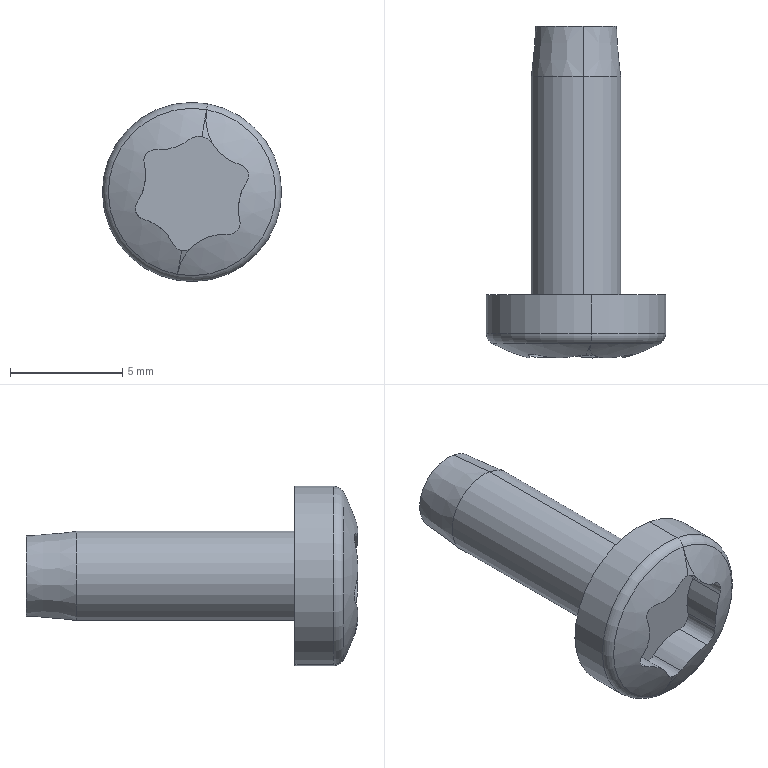Part | SolidWorks | features BaseBody 1 | 1 solid | 27 faces | box 8 x 14.81 x 8 mm | volume 243.858 mm3 | cylinder 16 | sphere 4 | plane 3 | torus 2 | cone 2 | commonest cylinder face diameters 4.272 x6 1 x5 4 x2 8 x2 1.5 x1
STEP:
#1=CARTESIAN_POINT('',(2057.198,-49.401,812.67));
#2=VERTEX_POINT('',#1);
#3=CARTESIAN_POINT('',(2056.608,-49.458,812.525));
#4=VERTEX_POINT('',#3);
#5=CARTESIAN_POINT('',(2057.198,-49.401,812.67));
#6=CARTESIAN_POINT('',(2057.147,-49.401,812.679));
#7=CARTESIAN_POINT('',(2057.043,-49.404,812.687));
#8=CARTESIAN_POINT('',(2056.888,-49.415,812.666));
#9=CARTESIAN_POINT('',(2056.74,-49.433,812.613));
#10=CARTESIAN_POINT('',(2056.65,-49.449,812.558));
#11=CARTESIAN_POINT('',(2056.608,-49.458,812.525));
#12=B_SPLINE_CURVE_WITH_KNOTS('',3,(#5,#6,#7,#8,#9,#10,#11),.UNSPECIFIED.,.F.,.F.,(4,1,1,1,4),(0.5,0.625,0.75,0.875,1.),.UNSPECIFIED.);
#13=EDGE_CURVE('',#2,#4,#12,.T.);
#14=ORIENTED_EDGE('',*,*,#13,.F.);
#15=CARTESIAN_POINT('',(2057.406,-48.898,813.843));
#16=VERTEX_POINT('',#15);
#17=CARTESIAN_POINT('',(2056.759,-41.805,810.2));
#18=DIRECTION('',(-0.9846,0.,0.1747));
#19=DIRECTION('',(0.1747,0.,0.9846));
#20=AXIS2_PLACEMENT_3D('',#17,#18,#19);
#21=CIRCLE('',#20,8.);
#22=EDGE_CURVE('',#2,#16,#21,.T.);
#23=ORIENTED_EDGE('',*,*,#22,.T.);
#24=CARTESIAN_POINT('',(2057.412,-48.88,813.876));
#25=VERTEX_POINT('',#24);
#26=CARTESIAN_POINT('',(2056.759,-41.805,810.2));
#27=DIRECTION('',(0.9846,0.,-0.1747));
#28=DIRECTION('',(0.08155,-0.8844,0.4595));
#29=AXIS2_PLACEMENT_3D('',#26,#27,#28);
#30=CIRCLE('',#29,8.);
#31=EDGE_CURVE('',#25,#16,#30,.T.);
#32=ORIENTED_EDGE('',*,*,#31,.F.);
#33=CARTESIAN_POINT('',(2056.107,-48.88,806.524));
#34=VERTEX_POINT('',#33);
#35=CARTESIAN_POINT('',(2056.759,-48.88,810.2));
#36=DIRECTION('',(0.,1.,0.));
#37=DIRECTION('',(-0.1747,0.,-0.9846));
#38=AXIS2_PLACEMENT_3D('',#35,#36,#37);
#39=CIRCLE('',#38,3.733);
#40=EDGE_CURVE('',#34,#25,#39,.T.);
#41=ORIENTED_EDGE('',*,*,#40,.F.);
#42=CARTESIAN_POINT('',(2056.113,-48.898,806.557));
#43=VERTEX_POINT('',#42);
#44=CARTESIAN_POINT('',(2056.759,-41.805,810.2));
#45=DIRECTION('',(0.9846,0.,-0.1747));
#46=DIRECTION('',(-0.08155,-0.8844,-0.4595));
#47=AXIS2_PLACEMENT_3D('',#44,#45,#46);
#48=CIRCLE('',#47,8.);
#49=EDGE_CURVE('',#43,#34,#48,.T.);
#50=ORIENTED_EDGE('',*,*,#49,.F.);
#51=CARTESIAN_POINT('',(2056.295,-49.351,807.585));
#52=VERTEX_POINT('',#51);
#53=CARTESIAN_POINT('',(2056.759,-41.805,810.2));
#54=DIRECTION('',(0.9846,0.,-0.1747));
#55=DIRECTION('',(-0.1747,0.,-0.9846));
#56=AXIS2_PLACEMENT_3D('',#53,#54,#55);
#57=CIRCLE('',#56,8.);
#58=EDGE_CURVE('',#52,#43,#57,.T.);
#59=ORIENTED_EDGE('',*,*,#58,.F.);
#60=CARTESIAN_POINT('',(2055.933,-49.41,807.86));
#61=VERTEX_POINT('',#60);
#62=CARTESIAN_POINT('',(2056.295,-49.351,807.585));
#63=CARTESIAN_POINT('',(2056.257,-49.351,807.592));
#64=CARTESIAN_POINT('',(2056.182,-49.354,807.615));
#65=CARTESIAN_POINT('',(2056.08,-49.366,807.674));
#66=CARTESIAN_POINT('',(2055.994,-49.384,807.756));
#67=CARTESIAN_POINT('',(2055.95,-49.401,807.824));
#68=CARTESIAN_POINT('',(2055.933,-49.41,807.86));
#69=B_SPLINE_CURVE_WITH_KNOTS('',3,(#62,#63,#64,#65,#66,#67,#68),.UNSPECIFIED.,.F.,.F.,(4,1,1,1,4),(0.5,0.625,0.75,0.875,1.),.UNSPECIFIED.);
#70=EDGE_CURVE('',#52,#61,#69,.T.);
#71=ORIENTED_EDGE('',*,*,#70,.T.);
#72=CARTESIAN_POINT('',(2054.596,-49.41,808.984));
#73=VERTEX_POINT('',#72);
#74=CARTESIAN_POINT('',(2055.933,-49.41,807.86));
#75=CARTESIAN_POINT('',(2055.868,-49.445,807.994));
#76=CARTESIAN_POINT('',(2055.79,-49.47,808.12));
#77=CARTESIAN_POINT('',(2055.606,-49.505,808.357));
#78=CARTESIAN_POINT('',(2055.5,-49.514,808.468));
#79=CARTESIAN_POINT('',(2055.27,-49.515,808.661));
#80=CARTESIAN_POINT('',(2055.144,-49.506,808.746));
#81=CARTESIAN_POINT('',(2054.877,-49.47,808.888));
#82=CARTESIAN_POINT('',(2054.739,-49.445,808.943));
#83=CARTESIAN_POINT('',(2054.596,-49.41,808.984));
#84=B_SPLINE_CURVE_WITH_KNOTS('',3,(#74,#75,#76,#77,#78,#79,#80,#81,#82,#83),.UNSPECIFIED.,.F.,.F.,(4,2,2,2,4),(0.,0.0004513,0.0009026,0.001354,0.001805),.UNSPECIFIED.);
#85=EDGE_CURVE('',#61,#73,#84,.T.);
#86=ORIENTED_EDGE('',*,*,#85,.T.);
#87=CARTESIAN_POINT('',(2054.32,-49.41,809.746));
#88=VERTEX_POINT('',#87);
#89=CARTESIAN_POINT('',(2054.596,-49.41,808.984));
#90=CARTESIAN_POINT('',(2054.557,-49.401,808.995));
#91=CARTESIAN_POINT('',(2054.483,-49.384,809.026));
#92=CARTESIAN_POINT('',(2054.388,-49.366,809.097));
#93=CARTESIAN_POINT('',(2054.312,-49.354,809.188));
#94=CARTESIAN_POINT('',(2054.259,-49.35,809.293));
#95=CARTESIAN_POINT('',(2054.232,-49.354,809.407));
#96=CARTESIAN_POINT('',(2054.232,-49.366,809.526));
#97=CARTESIAN_POINT('',(2054.26,-49.384,809.641));
#98=CARTESIAN_POINT('',(2054.297,-49.401,809.713));
#99=CARTESIAN_POINT('',(2054.32,-49.41,809.746));
#100=B_SPLINE_CURVE_WITH_KNOTS('',3,(#89,#90,#91,#92,#93,#94,#95,#96,#97,#98,#99),.UNSPECIFIED.,.F.,.F.,(4,1,1,1,1,1,1,1,4),(0.,0.125,0.25,0.375,0.5,0.625,0.75,0.875,1.),.UNSPECIFIED.);
#101=EDGE_CURVE('',#73,#88,#100,.T.);
#102=ORIENTED_EDGE('',*,*,#101,.T.);
#103=CARTESIAN_POINT('',(2054.625,-49.41,811.465));
#104=VERTEX_POINT('',#103);
#105=CARTESIAN_POINT('',(2054.32,-49.41,809.746));
#106=CARTESIAN_POINT('',(2054.403,-49.445,809.869));
#107=CARTESIAN_POINT('',(2054.473,-49.47,810.));
#108=CARTESIAN_POINT('',(2054.587,-49.505,810.277));
#109=CARTESIAN_POINT('',(2054.63,-49.514,810.424));
#110=CARTESIAN_POINT('',(2054.682,-49.515,810.721));
#111=CARTESIAN_POINT('',(2054.693,-49.506,810.872));
#112=CARTESIAN_POINT('',(2054.682,-49.47,811.174));
#113=CARTESIAN_POINT('',(2054.661,-49.445,811.321));
#114=CARTESIAN_POINT('',(2054.625,-49.41,811.465));
#115=B_SPLINE_CURVE_WITH_KNOTS('',3,(#105,#106,#107,#108,#109,#110,#111,#112,#113,#114),.UNSPECIFIED.,.F.,.F.,(4,2,2,2,4),(0.,0.0004513,0.0009026,0.001354,0.001805),.UNSPECIFIED.);
#116=EDGE_CURVE('',#88,#104,#115,.T.);
#117=ORIENTED_EDGE('',*,*,#116,.T.);
#118=CARTESIAN_POINT('',(2055.146,-49.41,812.086));
#119=VERTEX_POINT('',#118);
#120=CARTESIAN_POINT('',(2054.625,-49.41,811.465));
#121=CARTESIAN_POINT('',(2054.615,-49.401,811.504));
#122=CARTESIAN_POINT('',(2054.605,-49.384,811.584));
#123=CARTESIAN_POINT('',(2054.619,-49.366,811.702));
#124=CARTESIAN_POINT('',(2054.659,-49.354,811.813));
#125=CARTESIAN_POINT('',(2054.724,-49.35,811.912));
#126=CARTESIAN_POINT('',(2054.81,-49.354,811.992));
#127=CARTESIAN_POINT('',(2054.912,-49.366,812.051));
#128=CARTESIAN_POINT('',(2055.026,-49.384,812.085));
#129=CARTESIAN_POINT('',(2055.106,-49.401,812.089));
#130=CARTESIAN_POINT('',(2055.146,-49.41,812.086));
#131=B_SPLINE_CURVE_WITH_KNOTS('',3,(#120,#121,#122,#123,#124,#125,#126,#127,#128,#129,#130),.UNSPECIFIED.,.F.,.F.,(4,1,1,1,1,1,1,1,4),(0.,0.125,0.25,0.375,0.5,0.625,0.75,0.875,1.),.UNSPECIFIED.);
#132=EDGE_CURVE('',#104,#119,#131,.T.);
#133=ORIENTED_EDGE('',*,*,#132,.T.);
#134=CARTESIAN_POINT('',(2055.146,-49.41,812.086));
#135=CARTESIAN_POINT('',(2055.215,-49.426,812.081));
#136=CARTESIAN_POINT('',(2055.35,-49.454,812.077));
#137=CARTESIAN_POINT('',(2055.547,-49.484,812.091));
#138=CARTESIAN_POINT('',(2055.738,-49.504,812.122));
#139=CARTESIAN_POINT('',(2055.925,-49.514,812.17));
#140=CARTESIAN_POINT('',(2056.108,-49.515,812.234));
#141=CARTESIAN_POINT('',(2056.283,-49.506,812.315));
#142=CARTESIAN_POINT('',(2056.45,-49.488,812.411));
#143=CARTESIAN_POINT('',(2056.557,-49.469,812.486));
#144=CARTESIAN_POINT('',(2056.608,-49.458,812.525));
#145=B_SPLINE_CURVE_WITH_KNOTS('',3,(#134,#135,#136,#137,#138,#139,#140,#141,#142,#143,#144),.UNSPECIFIED.,.F.,.F.,(4,1,1,1,1,1,1,1,4),(0.,0.125,0.25,0.375,0.5,0.625,0.75,0.875,1.),.UNSPECIFIED.);
#146=EDGE_CURVE('',#119,#4,#145,.T.);
#147=ORIENTED_EDGE('',*,*,#146,.T.);
#148=EDGE_LOOP('',(#14,#23,#32,#41,#50,#59,#71,#86,#102,#117,#133,#147));
#149=FACE_OUTER_BOUND('',#148,.T.);
#150=CARTESIAN_POINT('',(2056.759,-41.805,810.2));
#151=DIRECTION('',(-0.9846,0.,0.1747));
#152=DIRECTION('',(-0.1747,0.,-0.9846));
#153=AXIS2_PLACEMENT_3D('',#150,#151,#152);
#154=SPHERICAL_SURFACE('',#153,8.);
#155=ADVANCED_FACE('',(#149),#154,.T.);
#156=CARTESIAN_POINT('',(2056.73,-49.41,807.718));
#157=VERTEX_POINT('',#156);
#158=CARTESIAN_POINT('',(2056.73,-49.41,807.718));
#159=CARTESIAN_POINT('',(2056.702,-49.401,807.69));
#160=CARTESIAN_POINT('',(2056.638,-49.384,807.642));
#161=CARTESIAN_POINT('',(2056.529,-49.366,807.595));
#162=CARTESIAN_POINT('',(2056.412,-49.354,807.574));
#163=CARTESIAN_POINT('',(2056.334,-49.351,807.579));
#164=CARTESIAN_POINT('',(2056.295,-49.351,807.585));
#165=B_SPLINE_CURVE_WITH_KNOTS('',3,(#158,#159,#160,#161,#162,#163,#164),.UNSPECIFIED.,.F.,.F.,(4,1,1,1,4),(0.,0.125,0.25,0.375,0.5),.UNSPECIFIED.);
#166=EDGE_CURVE('',#157,#52,#165,.T.);
#167=ORIENTED_EDGE('',*,*,#166,.T.);
#168=ORIENTED_EDGE('',*,*,#58,.T.);
#169=CARTESIAN_POINT('',(2056.73,-49.41,807.718));
#170=CARTESIAN_POINT('',(2056.679,-49.394,807.669));
#171=CARTESIAN_POINT('',(2056.578,-49.356,807.561));
#172=CARTESIAN_POINT('',(2056.434,-49.282,807.37));
#173=CARTESIAN_POINT('',(2056.3,-49.185,807.141));
#174=CARTESIAN_POINT('',(2056.186,-49.06,806.872));
#175=CARTESIAN_POINT('',(2056.132,-48.956,806.666));
#176=CARTESIAN_POINT('',(2056.113,-48.898,806.557));
#177=B_SPLINE_CURVE_WITH_KNOTS('',3,(#169,#170,#171,#172,#173,#174,#175,#176),.UNSPECIFIED.,.F.,.F.,(4,1,1,1,1,4),(0.,0.2,0.4,0.6,0.8,1.),.UNSPECIFIED.);
#178=EDGE_CURVE('',#157,#43,#177,.T.);
#179=ORIENTED_EDGE('',*,*,#178,.F.);
#180=EDGE_LOOP('',(#167,#168,#179));
#181=FACE_OUTER_BOUND('',#180,.T.);
#182=CARTESIAN_POINT('',(2056.759,-41.805,810.2));
#183=DIRECTION('',(-0.9846,0.,0.1747));
#184=DIRECTION('',(-0.1747,0.,-0.9846));
#185=AXIS2_PLACEMENT_3D('',#182,#183,#184);
#186=SPHERICAL_SURFACE('',#185,8.);
#187=ADVANCED_FACE('',(#181),#186,.T.);
#188=CARTESIAN_POINT('',(2056.06,-46.705,806.261));
#189=VERTEX_POINT('',#188);
#190=CARTESIAN_POINT('',(2057.458,-46.705,814.138));
#191=VERTEX_POINT('',#190);
#192=CARTESIAN_POINT('',(2056.759,-46.705,810.2));
#193=DIRECTION('',(0.,-1.,0.));
#194=DIRECTION('',(-0.1747,0.,-0.9846));
#195=AXIS2_PLACEMENT_3D('',#192,#193,#194);
#196=CIRCLE('',#195,4.);
#197=EDGE_CURVE('',#189,#191,#196,.T.);
#198=ORIENTED_EDGE('',*,*,#197,.F.);
#199=CARTESIAN_POINT('',(2056.759,-46.705,810.2));
#200=DIRECTION('',(0.,1.,0.));
#201=DIRECTION('',(-0.1747,0.,-0.9846));
#202=AXIS2_PLACEMENT_3D('',#199,#200,#201);
#203=CIRCLE('',#202,4.);
#204=EDGE_CURVE('',#189,#191,#203,.T.);
#205=ORIENTED_EDGE('',*,*,#204,.T.);
#206=EDGE_LOOP('',(#198,#205));
#207=FACE_OUTER_BOUND('',#206,.T.);
#208=CARTESIAN_POINT('',(2056.41,-46.705,808.231));
#209=VERTEX_POINT('',#208);
#210=CARTESIAN_POINT('',(2057.109,-46.705,812.169));
#211=VERTEX_POINT('',#210);
#212=CARTESIAN_POINT('',(2056.759,-46.705,810.2));
#213=DIRECTION('',(0.,1.,0.));
#214=DIRECTION('',(-0.1747,0.,-0.9846));
#215=AXIS2_PLACEMENT_3D('',#212,#213,#214);
#216=CIRCLE('',#215,2.);
#217=EDGE_CURVE('',#209,#211,#216,.T.);
#218=ORIENTED_EDGE('',*,*,#217,.F.);
#219=CARTESIAN_POINT('',(2056.759,-46.705,810.2));
#220=DIRECTION('',(0.,-1.,0.));
#221=DIRECTION('',(-0.1747,0.,-0.9846));
#222=AXIS2_PLACEMENT_3D('',#219,#220,#221);
#223=CIRCLE('',#222,2.);
#224=EDGE_CURVE('',#209,#211,#223,.T.);
#225=ORIENTED_EDGE('',*,*,#224,.T.);
#226=EDGE_LOOP('',(#218,#225));
#227=FACE_BOUND('',#226,.T.);
#228=CARTESIAN_POINT('',(2056.759,-46.705,810.2));
#229=DIRECTION('',(0.,1.,0.));
#230=DIRECTION('',(-0.1747,0.,-0.9846));
#231=AXIS2_PLACEMENT_3D('',#228,#229,#230);
#232=PLANE('',#231);
#233=ADVANCED_FACE('',(#207,#227),#232,.T.);
#234=CARTESIAN_POINT('',(2056.06,-48.438,806.261));
#235=VERTEX_POINT('',#234);
#236=CARTESIAN_POINT('',(2057.458,-48.438,814.138));
#237=VERTEX_POINT('',#236);
#238=CARTESIAN_POINT('',(2056.759,-48.438,810.2));
#239=DIRECTION('',(0.,1.,0.));
#240=DIRECTION('',(-0.1747,0.,-0.9846));
#241=AXIS2_PLACEMENT_3D('',#238,#239,#240);
#242=CIRCLE('',#241,4.);
#243=EDGE_CURVE('',#235,#237,#242,.T.);
#244=ORIENTED_EDGE('',*,*,#243,.T.);
#245=CARTESIAN_POINT('',(2057.458,-46.705,814.138));
#246=DIRECTION('',(0.,1.,0.));
#247=VECTOR('',#246,1000.);
#248=LINE('',#245,#247);
#249=EDGE_CURVE('',#237,#191,#248,.T.);
#250=ORIENTED_EDGE('',*,*,#249,.T.);
#251=ORIENTED_EDGE('',*,*,#204,.F.);
#252=CARTESIAN_POINT('',(2056.06,-46.705,806.261));
#253=DIRECTION('',(0.,-1.,0.));
#254=VECTOR('',#253,1000.);
#255=LINE('',#252,#254);
#256=EDGE_CURVE('',#189,#235,#255,.T.);
#257=ORIENTED_EDGE('',*,*,#256,.T.);
#258=EDGE_LOOP('',(#244,#250,#251,#257));
#259=FACE_OUTER_BOUND('',#258,.T.);
#260=CARTESIAN_POINT('',(2056.759,-50.56,810.2));
#261=DIRECTION('',(0.,1.,0.));
#262=DIRECTION('',(-0.1747,0.,-0.9846));
#263=AXIS2_PLACEMENT_3D('',#260,#261,#262);
#264=CYLINDRICAL_SURFACE('',#263,4.);
#265=ADVANCED_FACE('',(#259),#264,.T.);
#266=ORIENTED_EDGE('',*,*,#197,.T.);
#267=ORIENTED_EDGE('',*,*,#249,.F.);
#268=CARTESIAN_POINT('',(2056.759,-48.438,810.2));
#269=DIRECTION('',(0.,-1.,0.));
#270=DIRECTION('',(-0.1747,0.,-0.9846));
#271=AXIS2_PLACEMENT_3D('',#268,#269,#270);
#272=CIRCLE('',#271,4.);
#273=EDGE_CURVE('',#235,#237,#272,.T.);
#274=ORIENTED_EDGE('',*,*,#273,.F.);
#275=ORIENTED_EDGE('',*,*,#256,.F.);
#276=EDGE_LOOP('',(#266,#267,#274,#275));
#277=FACE_OUTER_BOUND('',#276,.T.);
#278=CARTESIAN_POINT('',(2056.759,-50.56,810.2));
#279=DIRECTION('',(0.,1.,0.));
#280=DIRECTION('',(-0.1747,0.,-0.9846));
#281=AXIS2_PLACEMENT_3D('',#278,#279,#280);
#282=CYLINDRICAL_SURFACE('',#281,4.);
#283=ADVANCED_FACE('',(#277),#282,.T.);
#284=ORIENTED_EDGE('',*,*,#273,.T.);
#285=CARTESIAN_POINT('',(2057.371,-48.438,813.646));
#286=DIRECTION('',(-0.9846,0.,0.1747));
#287=DIRECTION('',(0.1747,0.,0.9846));
#288=AXIS2_PLACEMENT_3D('',#285,#286,#287);
#289=CIRCLE('',#288,0.5);
#290=EDGE_CURVE('',#25,#237,#289,.T.);
#291=ORIENTED_EDGE('',*,*,#290,.F.);
#292=CARTESIAN_POINT('',(2056.759,-48.88,810.2));
#293=DIRECTION('',(0.,-1.,0.));
#294=DIRECTION('',(-0.1747,0.,-0.9846));
#295=AXIS2_PLACEMENT_3D('',#292,#293,#294);
#296=CIRCLE('',#295,3.733);
#297=EDGE_CURVE('',#34,#25,#296,.T.);
#298=ORIENTED_EDGE('',*,*,#297,.F.);
#299=CARTESIAN_POINT('',(2056.148,-48.438,806.754));
#300=DIRECTION('',(-0.9846,0.,0.1747));
#301=DIRECTION('',(-0.1747,0.,-0.9846));
#302=AXIS2_PLACEMENT_3D('',#299,#300,#301);
#303=CIRCLE('',#302,0.5);
#304=EDGE_CURVE('',#235,#34,#303,.T.);
#305=ORIENTED_EDGE('',*,*,#304,.F.);
#306=EDGE_LOOP('',(#284,#291,#298,#305));
#307=FACE_OUTER_BOUND('',#306,.T.);
#308=CARTESIAN_POINT('',(2056.759,-48.438,810.2));
#309=DIRECTION('',(0.,1.,0.));
#310=DIRECTION('',(-0.1747,0.,-0.9846));
#311=AXIS2_PLACEMENT_3D('',#308,#309,#310);
#312=TOROIDAL_SURFACE('',#311,3.5,0.5);
#313=ADVANCED_FACE('',(#307),#312,.T.);
#314=ORIENTED_EDGE('',*,*,#40,.T.);
#315=ORIENTED_EDGE('',*,*,#290,.T.);
#316=ORIENTED_EDGE('',*,*,#243,.F.);
#317=ORIENTED_EDGE('',*,*,#304,.T.);
#318=EDGE_LOOP('',(#314,#315,#316,#317));
#319=FACE_OUTER_BOUND('',#318,.T.);
#320=CARTESIAN_POINT('',(2056.759,-48.438,810.2));
#321=DIRECTION('',(0.,1.,0.));
#322=DIRECTION('',(-0.1747,0.,-0.9846));
#323=AXIS2_PLACEMENT_3D('',#320,#321,#322);
#324=TOROIDAL_SURFACE('',#323,3.5,0.5);
#325=ADVANCED_FACE('',(#319),#324,.T.);
#326=ORIENTED_EDGE('',*,*,#22,.F.);
#327=CARTESIAN_POINT('',(2057.701,-49.458,812.331));
#328=VERTEX_POINT('',#327);
#329=CARTESIAN_POINT('',(2057.701,-49.458,812.331));
#330=CARTESIAN_POINT('',(2057.673,-49.449,812.376));
#331=CARTESIAN_POINT('',(2057.608,-49.433,812.459));
#332=CARTESIAN_POINT('',(2057.487,-49.415,812.559));
#333=CARTESIAN_POINT('',(2057.349,-49.404,812.633));
#334=CARTESIAN_POINT('',(2057.249,-49.401,812.661));
#335=CARTESIAN_POINT('',(2057.198,-49.401,812.67));
#336=B_SPLINE_CURVE_WITH_KNOTS('',3,(#329,#330,#331,#332,#333,#334,#335),.UNSPECIFIED.,.F.,.F.,(4,1,1,1,4),(0.,0.125,0.25,0.375,0.5),.UNSPECIFIED.);
#337=EDGE_CURVE('',#328,#2,#336,.T.);
#338=ORIENTED_EDGE('',*,*,#337,.F.);
#339=CARTESIAN_POINT('',(2057.406,-48.898,813.843));
#340=CARTESIAN_POINT('',(2057.387,-48.953,813.738));
#341=CARTESIAN_POINT('',(2057.367,-49.054,813.534));
#342=CARTESIAN_POINT('',(2057.379,-49.179,813.244));
#343=CARTESIAN_POINT('',(2057.425,-49.279,812.979));
#344=CARTESIAN_POINT('',(2057.496,-49.356,812.741));
#345=CARTESIAN_POINT('',(2057.59,-49.416,812.522));
#346=CARTESIAN_POINT('',(2057.662,-49.446,812.393));
#347=CARTESIAN_POINT('',(2057.701,-49.458,812.331));
#348=B_SPLINE_CURVE_WITH_KNOTS('',3,(#339,#340,#341,#342,#343,#344,#345,#346,#347),.UNSPECIFIED.,.F.,.F.,(4,1,1,1,1,1,4),(0.,0.1667,0.3333,0.5,0.6667,0.8333,1.),.UNSPECIFIED.);
#349=EDGE_CURVE('',#16,#328,#348,.T.);
#350=ORIENTED_EDGE('',*,*,#349,.F.);
#351=EDGE_LOOP('',(#326,#338,#350));
#352=FACE_OUTER_BOUND('',#351,.T.);
#353=CARTESIAN_POINT('',(2056.759,-41.805,810.2));
#354=DIRECTION('',(-0.9846,0.,0.1747));
#355=DIRECTION('',(-0.1747,0.,-0.9846));
#356=AXIS2_PLACEMENT_3D('',#353,#354,#355);
#357=SPHERICAL_SURFACE('',#356,8.);
#358=ADVANCED_FACE('',(#352),#357,.T.);
#359=CARTESIAN_POINT('',(2054.32,-47.705,809.746));
#360=VERTEX_POINT('',#359);
#361=CARTESIAN_POINT('',(2054.625,-47.705,811.465));
#362=VERTEX_POINT('',#361);
#363=CARTESIAN_POINT('',(2052.553,-47.705,810.946));
#364=DIRECTION('',(0.,-1.,0.));
#365=DIRECTION('',(0.8272,0.,-0.562));
#366=AXIS2_PLACEMENT_3D('',#363,#364,#365);
#367=CIRCLE('',#366,2.136);
#368=EDGE_CURVE('',#360,#362,#367,.T.);
#369=ORIENTED_EDGE('',*,*,#368,.T.);
#370=CARTESIAN_POINT('',(2054.625,-49.41,811.465));
#371=DIRECTION('',(0.,1.,0.));
#372=VECTOR('',#371,1000.);
#373=LINE('',#370,#372);
#374=EDGE_CURVE('',#104,#362,#373,.T.);
#375=ORIENTED_EDGE('',*,*,#374,.F.);
#376=ORIENTED_EDGE('',*,*,#116,.F.);
#377=CARTESIAN_POINT('',(2054.32,-49.41,809.746));
#378=DIRECTION('',(0.,1.,0.));
#379=VECTOR('',#378,1000.);
#380=LINE('',#377,#379);
#381=EDGE_CURVE('',#88,#360,#380,.T.);
#382=ORIENTED_EDGE('',*,*,#381,.T.);
#383=EDGE_LOOP('',(#369,#375,#376,#382));
#384=FACE_OUTER_BOUND('',#383,.T.);
#385=CARTESIAN_POINT('',(2052.553,-47.705,810.946));
#386=DIRECTION('',(0.,1.,0.));
#387=DIRECTION('',(-0.1747,0.,-0.9846));
#388=AXIS2_PLACEMENT_3D('',#385,#386,#387);
#389=CYLINDRICAL_SURFACE('',#388,2.136);
#390=ADVANCED_FACE('',(#384),#389,.T.);
#391=CARTESIAN_POINT('',(2054.596,-47.705,808.984));
#392=VERTEX_POINT('',#391);
#393=CARTESIAN_POINT('',(2054.733,-47.705,809.465));
#394=DIRECTION('',(0.,1.,0.));
#395=DIRECTION('',(-0.2746,0.,-0.9616));
#396=AXIS2_PLACEMENT_3D('',#393,#394,#395);
#397=CIRCLE('',#396,0.5);
#398=EDGE_CURVE('',#392,#360,#397,.T.);
#399=ORIENTED_EDGE('',*,*,#398,.T.);
#400=ORIENTED_EDGE('',*,*,#381,.F.);
#401=ORIENTED_EDGE('',*,*,#101,.F.);
#402=CARTESIAN_POINT('',(2054.596,-49.41,808.984));
#403=DIRECTION('',(0.,1.,0.));
#404=VECTOR('',#403,1000.);
#405=LINE('',#402,#404);
#406=EDGE_CURVE('',#73,#392,#405,.T.);
#407=ORIENTED_EDGE('',*,*,#406,.T.);
#408=EDGE_LOOP('',(#399,#400,#401,#407));
#409=FACE_OUTER_BOUND('',#408,.T.);
#410=CARTESIAN_POINT('',(2054.733,-50.419,809.465));
#411=DIRECTION('',(0.,1.,0.));
#412=DIRECTION('',(0.8272,0.,-0.562));
#413=AXIS2_PLACEMENT_3D('',#410,#411,#412);
#414=CYLINDRICAL_SURFACE('',#413,0.5);
#415=ADVANCED_FACE('',(#409),#414,.F.);
#416=ORIENTED_EDGE('',*,*,#85,.F.);
#417=CARTESIAN_POINT('',(2055.933,-47.705,807.86));
#418=VERTEX_POINT('',#417);
#419=CARTESIAN_POINT('',(2055.933,-49.41,807.86));
#420=DIRECTION('',(0.,1.,0.));
#421=VECTOR('',#420,1000.);
#422=LINE('',#419,#421);
#423=EDGE_CURVE('',#61,#418,#422,.T.);
#424=ORIENTED_EDGE('',*,*,#423,.T.);
#425=CARTESIAN_POINT('',(2054.009,-47.705,806.93));
#426=DIRECTION('',(0.,-1.,0.));
#427=DIRECTION('',(0.9003,0.,0.4353));
#428=AXIS2_PLACEMENT_3D('',#425,#426,#427);
#429=CIRCLE('',#428,2.136);
#430=EDGE_CURVE('',#418,#392,#429,.T.);
#431=ORIENTED_EDGE('',*,*,#430,.T.);
#432=ORIENTED_EDGE('',*,*,#406,.F.);
#433=EDGE_LOOP('',(#416,#424,#431,#432));
#434=FACE_OUTER_BOUND('',#433,.T.);
#435=CARTESIAN_POINT('',(2054.009,-47.705,806.93));
#436=DIRECTION('',(0.,1.,0.));
#437=DIRECTION('',(-0.1747,0.,-0.9846));
#438=AXIS2_PLACEMENT_3D('',#435,#436,#437);
#439=CYLINDRICAL_SURFACE('',#438,2.136);
#440=ADVANCED_FACE('',(#434),#439,.T.);
#441=ORIENTED_EDGE('',*,*,#430,.F.);
#442=CARTESIAN_POINT('',(2056.73,-47.705,807.718));
#443=VERTEX_POINT('',#442);
#444=CARTESIAN_POINT('',(2056.383,-47.705,808.078));
#445=DIRECTION('',(0.,1.,0.));
#446=DIRECTION('',(0.6955,0.,-0.7186));
#447=AXIS2_PLACEMENT_3D('',#444,#445,#446);
#448=CIRCLE('',#447,0.5);
#449=EDGE_CURVE('',#443,#418,#448,.T.);
#450=ORIENTED_EDGE('',*,*,#449,.F.);
#451=CARTESIAN_POINT('',(2058.372,-47.705,808.314));
#452=VERTEX_POINT('',#451);
#453=CARTESIAN_POINT('',(2058.216,-47.705,806.183));
#454=DIRECTION('',(0.,-1.,0.));
#455=DIRECTION('',(0.07311,0.,0.9973));
#456=AXIS2_PLACEMENT_3D('',#453,#454,#455);
#457=CIRCLE('',#456,2.136);
#458=EDGE_CURVE('',#452,#443,#457,.T.);
#459=ORIENTED_EDGE('',*,*,#458,.F.);
#460=CARTESIAN_POINT('',(2058.894,-47.705,808.934));
#461=VERTEX_POINT('',#460);
#462=CARTESIAN_POINT('',(2058.409,-47.705,808.813));
#463=DIRECTION('',(0.,-1.,0.));
#464=DIRECTION('',(-0.07311,0.,-0.9973));
#465=AXIS2_PLACEMENT_3D('',#462,#463,#464);
#466=CIRCLE('',#465,0.5);
#467=EDGE_CURVE('',#452,#461,#466,.T.);
#468=ORIENTED_EDGE('',*,*,#467,.T.);
#469=CARTESIAN_POINT('',(2059.199,-47.705,810.654));
#470=VERTEX_POINT('',#469);
#471=CARTESIAN_POINT('',(2060.966,-47.705,809.453));
#472=DIRECTION('',(0.,-1.,0.));
#473=DIRECTION('',(-0.8272,0.,0.562));
#474=AXIS2_PLACEMENT_3D('',#471,#472,#473);
#475=CIRCLE('',#474,2.136);
#476=EDGE_CURVE('',#470,#461,#475,.T.);
#477=ORIENTED_EDGE('',*,*,#476,.F.);
#478=CARTESIAN_POINT('',(2058.923,-47.705,811.415));
#479=VERTEX_POINT('',#478);
#480=CARTESIAN_POINT('',(2058.785,-47.705,810.935));
#481=DIRECTION('',(0.,-1.,0.));
#482=DIRECTION('',(0.8272,0.,-0.562));
#483=AXIS2_PLACEMENT_3D('',#480,#481,#482);
#484=CIRCLE('',#483,0.5);
#485=EDGE_CURVE('',#470,#479,#484,.T.);
#486=ORIENTED_EDGE('',*,*,#485,.T.);
#487=CARTESIAN_POINT('',(2057.701,-47.705,812.331));
#488=VERTEX_POINT('',#487);
#489=CARTESIAN_POINT('',(2059.509,-47.705,813.47));
#490=DIRECTION('',(0.,-1.,0.));
#491=DIRECTION('',(-0.8463,0.,-0.5328));
#492=AXIS2_PLACEMENT_3D('',#489,#490,#491);
#493=CIRCLE('',#492,2.136);
#494=EDGE_CURVE('',#488,#479,#493,.T.);
#495=ORIENTED_EDGE('',*,*,#494,.F.);
#496=CARTESIAN_POINT('',(2056.608,-47.705,812.525));
#497=VERTEX_POINT('',#496);
#498=CARTESIAN_POINT('',(2057.067,-47.705,811.932));
#499=DIRECTION('',(0.,-1.,0.));
#500=DIRECTION('',(0.8463,0.,0.5328));
#501=AXIS2_PLACEMENT_3D('',#498,#499,#500);
#502=CIRCLE('',#501,0.75);
#503=EDGE_CURVE('',#488,#497,#502,.T.);
#504=ORIENTED_EDGE('',*,*,#503,.T.);
#505=CARTESIAN_POINT('',(2055.146,-47.705,812.086));
#506=VERTEX_POINT('',#505);
#507=CARTESIAN_POINT('',(2055.303,-47.705,814.216));
#508=DIRECTION('',(0.,-1.,0.));
#509=DIRECTION('',(-0.07311,0.,-0.9973));
#510=AXIS2_PLACEMENT_3D('',#507,#508,#509);
#511=CIRCLE('',#510,2.136);
#512=EDGE_CURVE('',#506,#497,#511,.T.);
#513=ORIENTED_EDGE('',*,*,#512,.F.);
#514=CARTESIAN_POINT('',(2055.11,-47.705,811.587));
#515=DIRECTION('',(0.,1.,0.));
#516=DIRECTION('',(-0.97,0.,-0.243));
#517=AXIS2_PLACEMENT_3D('',#514,#515,#516);
#518=CIRCLE('',#517,0.5);
#519=EDGE_CURVE('',#362,#506,#518,.T.);
#520=ORIENTED_EDGE('',*,*,#519,.F.);
#521=ORIENTED_EDGE('',*,*,#368,.F.);
#522=ORIENTED_EDGE('',*,*,#398,.F.);
#523=EDGE_LOOP('',(#441,#450,#459,#468,#477,#486,#495,#504,#513,#520,#521,#522));
#524=FACE_OUTER_BOUND('',#523,.T.);
#525=CARTESIAN_POINT('',(2056.759,-47.705,810.2));
#526=DIRECTION('',(0.,1.,0.));
#527=DIRECTION('',(-0.1747,0.,-0.9846));
#528=AXIS2_PLACEMENT_3D('',#525,#526,#527);
#529=PLANE('',#528);
#530=ADVANCED_FACE('',(#524),#529,.F.);
#531=ORIENTED_EDGE('',*,*,#519,.T.);
#532=CARTESIAN_POINT('',(2055.146,-49.41,812.086));
#533=DIRECTION('',(0.,1.,0.));
#534=VECTOR('',#533,1000.);
#535=LINE('',#532,#534);
#536=EDGE_CURVE('',#119,#506,#535,.T.);
#537=ORIENTED_EDGE('',*,*,#536,.F.);
#538=ORIENTED_EDGE('',*,*,#132,.F.);
#539=ORIENTED_EDGE('',*,*,#374,.T.);
#540=EDGE_LOOP('',(#531,#537,#538,#539));
#541=FACE_OUTER_BOUND('',#540,.T.);
#542=CARTESIAN_POINT('',(2055.11,-50.419,811.587));
#543=DIRECTION('',(0.,1.,0.));
#544=DIRECTION('',(-0.07311,0.,-0.9973));
#545=AXIS2_PLACEMENT_3D('',#542,#543,#544);
#546=CYLINDRICAL_SURFACE('',#545,0.5);
#547=ADVANCED_FACE('',(#541),#546,.F.);
#548=ORIENTED_EDGE('',*,*,#512,.T.);
#549=CARTESIAN_POINT('',(2056.608,-47.705,812.525));
#550=DIRECTION('',(0.,-1.,0.));
#551=VECTOR('',#550,1000.);
#552=LINE('',#549,#551);
#553=EDGE_CURVE('',#497,#4,#552,.T.);
#554=ORIENTED_EDGE('',*,*,#553,.T.);
#555=ORIENTED_EDGE('',*,*,#146,.F.);
#556=ORIENTED_EDGE('',*,*,#536,.T.);
#557=EDGE_LOOP('',(#548,#554,#555,#556));
#558=FACE_OUTER_BOUND('',#557,.T.);
#559=CARTESIAN_POINT('',(2055.303,-47.705,814.216));
#560=DIRECTION('',(0.,1.,0.));
#561=DIRECTION('',(-0.1747,0.,-0.9846));
#562=AXIS2_PLACEMENT_3D('',#559,#560,#561);
#563=CYLINDRICAL_SURFACE('',#562,2.136);
#564=ADVANCED_FACE('',(#558),#563,.T.);
#565=ORIENTED_EDGE('',*,*,#337,.T.);
#566=ORIENTED_EDGE('',*,*,#13,.T.);
#567=ORIENTED_EDGE('',*,*,#553,.F.);
#568=ORIENTED_EDGE('',*,*,#503,.F.);
#569=CARTESIAN_POINT('',(2057.701,-47.705,812.331));
#570=DIRECTION('',(-0.00001055,-1.,0.00001413));
#571=VECTOR('',#570,1000.);
#572=LINE('',#569,#571);
#573=EDGE_CURVE('',#488,#328,#572,.T.);
#574=ORIENTED_EDGE('',*,*,#573,.T.);
#575=EDGE_LOOP('',(#565,#566,#567,#568,#574));
#576=FACE_OUTER_BOUND('',#575,.T.);
#577=CARTESIAN_POINT('',(2057.067,-46.8,811.932));
#578=DIRECTION('',(0.,-1.,0.));
#579=DIRECTION('',(0.6112,0.,-0.7914));
#580=AXIS2_PLACEMENT_3D('',#577,#578,#579);
#581=CYLINDRICAL_SURFACE('',#580,0.75);
#582=ADVANCED_FACE('',(#576),#581,.F.);
#583=ORIENTED_EDGE('',*,*,#494,.T.);
#584=CARTESIAN_POINT('',(2058.923,-49.41,811.415));
#585=VERTEX_POINT('',#584);
#586=CARTESIAN_POINT('',(2058.923,-47.705,811.415));
#587=DIRECTION('',(0.,-1.,0.));
#588=VECTOR('',#587,1000.);
#589=LINE('',#586,#588);
#590=EDGE_CURVE('',#479,#585,#589,.T.);
#591=ORIENTED_EDGE('',*,*,#590,.T.);
#592=CARTESIAN_POINT('',(2057.701,-49.458,812.331));
#593=CARTESIAN_POINT('',(2057.736,-49.469,812.276));
#594=CARTESIAN_POINT('',(2057.811,-49.488,812.169));
#595=CARTESIAN_POINT('',(2057.935,-49.506,812.021));
#596=CARTESIAN_POINT('',(2058.072,-49.515,811.885));
#597=CARTESIAN_POINT('',(2058.221,-49.514,811.762));
#598=CARTESIAN_POINT('',(2058.38,-49.504,811.653));
#599=CARTESIAN_POINT('',(2058.549,-49.484,811.558));
#600=CARTESIAN_POINT('',(2058.729,-49.454,811.478));
#601=CARTESIAN_POINT('',(2058.857,-49.426,811.434));
#602=CARTESIAN_POINT('',(2058.923,-49.41,811.415));
#603=B_SPLINE_CURVE_WITH_KNOTS('',3,(#592,#593,#594,#595,#596,#597,#598,#599,#600,#601,#602),.UNSPECIFIED.,.F.,.F.,(4,1,1,1,1,1,1,1,4),(0.,0.125,0.25,0.375,0.5,0.625,0.75,0.875,1.),.UNSPECIFIED.);
#604=EDGE_CURVE('',#328,#585,#603,.T.);
#605=ORIENTED_EDGE('',*,*,#604,.F.);
#606=ORIENTED_EDGE('',*,*,#573,.F.);
#607=EDGE_LOOP('',(#583,#591,#605,#606));
#608=FACE_OUTER_BOUND('',#607,.T.);
#609=CARTESIAN_POINT('',(2059.509,-47.705,813.47));
#610=DIRECTION('',(0.,1.,0.));
#611=DIRECTION('',(-0.1747,0.,-0.9846));
#612=AXIS2_PLACEMENT_3D('',#609,#610,#611);
#613=CYLINDRICAL_SURFACE('',#612,2.136);
#614=ADVANCED_FACE('',(#608),#613,.T.);
#615=ORIENTED_EDGE('',*,*,#349,.T.);
#616=ORIENTED_EDGE('',*,*,#604,.T.);
#617=CARTESIAN_POINT('',(2059.199,-49.41,810.654));
#618=VERTEX_POINT('',#617);
#619=CARTESIAN_POINT('',(2059.199,-49.41,810.654));
#620=CARTESIAN_POINT('',(2059.222,-49.401,810.687));
#621=CARTESIAN_POINT('',(2059.258,-49.384,810.758));
#622=CARTESIAN_POINT('',(2059.286,-49.366,810.874));
#623=CARTESIAN_POINT('',(2059.287,-49.354,810.992));
#624=CARTESIAN_POINT('',(2059.26,-49.35,811.107));
#625=CARTESIAN_POINT('',(2059.207,-49.354,811.212));
#626=CARTESIAN_POINT('',(2059.131,-49.366,811.302));
#627=CARTESIAN_POINT('',(2059.035,-49.384,811.373));
#628=CARTESIAN_POINT('',(2058.961,-49.401,811.404));
#629=CARTESIAN_POINT('',(2058.923,-49.41,811.415));
#630=B_SPLINE_CURVE_WITH_KNOTS('',3,(#619,#620,#621,#622,#623,#624,#625,#626,#627,#628,#629),.UNSPECIFIED.,.F.,.F.,(4,1,1,1,1,1,1,1,4),(0.,0.125,0.25,0.375,0.5,0.625,0.75,0.875,1.),.UNSPECIFIED.);
#631=EDGE_CURVE('',#618,#585,#630,.T.);
#632=ORIENTED_EDGE('',*,*,#631,.F.);
#633=CARTESIAN_POINT('',(2058.894,-49.41,808.934));
#634=VERTEX_POINT('',#633);
#635=CARTESIAN_POINT('',(2059.199,-49.41,810.654));
#636=CARTESIAN_POINT('',(2059.116,-49.445,810.531));
#637=CARTESIAN_POINT('',(2059.045,-49.47,810.4));
#638=CARTESIAN_POINT('',(2058.932,-49.505,810.123));
#639=CARTESIAN_POINT('',(2058.889,-49.514,809.975));
#640=CARTESIAN_POINT('',(2058.836,-49.515,809.679));
#641=CARTESIAN_POINT('',(2058.826,-49.506,809.527));
#642=CARTESIAN_POINT('',(2058.837,-49.47,809.226));
#643=CARTESIAN_POINT('',(2058.858,-49.445,809.078));
#644=CARTESIAN_POINT('',(2058.894,-49.41,808.934));
#645=B_SPLINE_CURVE_WITH_KNOTS('',3,(#635,#636,#637,#638,#639,#640,#641,#642,#643,#644),.UNSPECIFIED.,.F.,.F.,(4,2,2,2,4),(0.,0.0004513,0.0009026,0.001354,0.001805),.UNSPECIFIED.);
#646=EDGE_CURVE('',#618,#634,#645,.T.);
#647=ORIENTED_EDGE('',*,*,#646,.T.);
#648=CARTESIAN_POINT('',(2058.372,-49.41,808.314));
#649=VERTEX_POINT('',#648);
#650=CARTESIAN_POINT('',(2058.372,-49.41,808.314));
#651=CARTESIAN_POINT('',(2058.412,-49.401,808.311));
#652=CARTESIAN_POINT('',(2058.493,-49.384,808.315));
#653=CARTESIAN_POINT('',(2058.607,-49.366,808.348));
#654=CARTESIAN_POINT('',(2058.709,-49.354,808.407));
#655=CARTESIAN_POINT('',(2058.795,-49.35,808.488));
#656=CARTESIAN_POINT('',(2058.86,-49.354,808.586));
#657=CARTESIAN_POINT('',(2058.9,-49.366,808.697));
#658=CARTESIAN_POINT('',(2058.914,-49.384,808.815));
#659=CARTESIAN_POINT('',(2058.904,-49.401,808.895));
#660=CARTESIAN_POINT('',(2058.894,-49.41,808.934));
#661=B_SPLINE_CURVE_WITH_KNOTS('',3,(#650,#651,#652,#653,#654,#655,#656,#657,#658,#659,#660),.UNSPECIFIED.,.F.,.F.,(4,1,1,1,1,1,1,1,4),(0.,0.125,0.25,0.375,0.5,0.625,0.75,0.875,1.),.UNSPECIFIED.);
#662=EDGE_CURVE('',#649,#634,#661,.T.);
#663=ORIENTED_EDGE('',*,*,#662,.F.);
#664=CARTESIAN_POINT('',(2058.372,-49.41,808.314));
#665=CARTESIAN_POINT('',(2058.224,-49.445,808.325));
#666=CARTESIAN_POINT('',(2058.076,-49.47,808.32));
#667=CARTESIAN_POINT('',(2057.779,-49.505,808.28));
#668=CARTESIAN_POINT('',(2057.63,-49.514,808.243));
#669=CARTESIAN_POINT('',(2057.347,-49.515,808.141));
#670=CARTESIAN_POINT('',(2057.21,-49.506,808.074));
#671=CARTESIAN_POINT('',(2056.954,-49.47,807.914));
#672=CARTESIAN_POINT('',(2056.837,-49.445,807.822));
#673=CARTESIAN_POINT('',(2056.73,-49.41,807.718));
#674=B_SPLINE_CURVE_WITH_KNOTS('',3,(#664,#665,#666,#667,#668,#669,#670,#671,#672,#673),.UNSPECIFIED.,.F.,.F.,(4,2,2,2,4),(0.,0.0004513,0.0009026,0.001354,0.001805),.UNSPECIFIED.);
#675=EDGE_CURVE('',#649,#157,#674,.T.);
#676=ORIENTED_EDGE('',*,*,#675,.T.);
#677=ORIENTED_EDGE('',*,*,#178,.T.);
#678=ORIENTED_EDGE('',*,*,#49,.T.);
#679=ORIENTED_EDGE('',*,*,#297,.T.);
#680=ORIENTED_EDGE('',*,*,#31,.T.);
#681=EDGE_LOOP('',(#615,#616,#632,#647,#663,#676,#677,#678,#679,#680));
#682=FACE_OUTER_BOUND('',#681,.T.);
#683=CARTESIAN_POINT('',(2056.759,-41.805,810.2));
#684=DIRECTION('',(-0.9846,0.,0.1747));
#685=DIRECTION('',(-0.1747,0.,-0.9846));
#686=AXIS2_PLACEMENT_3D('',#683,#684,#685);
#687=SPHERICAL_SURFACE('',#686,8.);
#688=ADVANCED_FACE('',(#682),#687,.T.);
#689=ORIENTED_EDGE('',*,*,#675,.F.);
#690=CARTESIAN_POINT('',(2058.372,-47.705,808.314));
#691=DIRECTION('',(0.,-1.,0.));
#692=VECTOR('',#691,1000.);
#693=LINE('',#690,#692);
#694=EDGE_CURVE('',#452,#649,#693,.T.);
#695=ORIENTED_EDGE('',*,*,#694,.F.);
#696=ORIENTED_EDGE('',*,*,#458,.T.);
#697=CARTESIAN_POINT('',(2056.73,-49.41,807.718));
#698=DIRECTION('',(0.000007459,1.,0.000005969));
#699=VECTOR('',#698,1000.);
#700=LINE('',#697,#699);
#701=EDGE_CURVE('',#157,#443,#700,.T.);
#702=ORIENTED_EDGE('',*,*,#701,.F.);
#703=EDGE_LOOP('',(#689,#695,#696,#702));
#704=FACE_OUTER_BOUND('',#703,.T.);
#705=CARTESIAN_POINT('',(2058.216,-47.705,806.183));
#706=DIRECTION('',(0.,1.,0.));
#707=DIRECTION('',(-0.1747,0.,-0.9846));
#708=AXIS2_PLACEMENT_3D('',#705,#706,#707);
#709=CYLINDRICAL_SURFACE('',#708,2.136);
#710=ADVANCED_FACE('',(#704),#709,.T.);
#711=ORIENTED_EDGE('',*,*,#449,.T.);
#712=ORIENTED_EDGE('',*,*,#423,.F.);
#713=ORIENTED_EDGE('',*,*,#70,.F.);
#714=ORIENTED_EDGE('',*,*,#166,.F.);
#715=ORIENTED_EDGE('',*,*,#701,.T.);
#716=EDGE_LOOP('',(#711,#712,#713,#714,#715));
#717=FACE_OUTER_BOUND('',#716,.T.);
#718=CARTESIAN_POINT('',(2056.383,-50.419,808.078));
#719=DIRECTION('',(0.,1.,0.));
#720=DIRECTION('',(0.9003,0.,0.4353));
#721=AXIS2_PLACEMENT_3D('',#718,#719,#720);
#722=CYLINDRICAL_SURFACE('',#721,0.5);
#723=ADVANCED_FACE('',(#717),#722,.F.);
#724=ORIENTED_EDGE('',*,*,#662,.T.);
#725=CARTESIAN_POINT('',(2058.894,-47.705,808.934));
#726=DIRECTION('',(0.,-1.,0.));
#727=VECTOR('',#726,1000.);
#728=LINE('',#725,#727);
#729=EDGE_CURVE('',#461,#634,#728,.T.);
#730=ORIENTED_EDGE('',*,*,#729,.F.);
#731=ORIENTED_EDGE('',*,*,#467,.F.);
#732=ORIENTED_EDGE('',*,*,#694,.T.);
#733=EDGE_LOOP('',(#724,#730,#731,#732));
#734=FACE_OUTER_BOUND('',#733,.T.);
#735=CARTESIAN_POINT('',(2058.409,-46.8,808.813));
#736=DIRECTION('',(0.,-1.,0.));
#737=DIRECTION('',(-0.97,0.,-0.243));
#738=AXIS2_PLACEMENT_3D('',#735,#736,#737);
#739=CYLINDRICAL_SURFACE('',#738,0.5);
#740=ADVANCED_FACE('',(#734),#739,.F.);
#741=ORIENTED_EDGE('',*,*,#476,.T.);
#742=ORIENTED_EDGE('',*,*,#729,.T.);
#743=ORIENTED_EDGE('',*,*,#646,.F.);
#744=CARTESIAN_POINT('',(2059.199,-47.705,810.654));
#745=DIRECTION('',(0.,-1.,0.));
#746=VECTOR('',#745,1000.);
#747=LINE('',#744,#746);
#748=EDGE_CURVE('',#470,#618,#747,.T.);
#749=ORIENTED_EDGE('',*,*,#748,.F.);
#750=EDGE_LOOP('',(#741,#742,#743,#749));
#751=FACE_OUTER_BOUND('',#750,.T.);
#752=CARTESIAN_POINT('',(2060.966,-47.705,809.453));
#753=DIRECTION('',(0.,1.,0.));
#754=DIRECTION('',(-0.1747,0.,-0.9846));
#755=AXIS2_PLACEMENT_3D('',#752,#753,#754);
#756=CYLINDRICAL_SURFACE('',#755,2.136);
#757=ADVANCED_FACE('',(#751),#756,.T.);
#758=ORIENTED_EDGE('',*,*,#631,.T.);
#759=ORIENTED_EDGE('',*,*,#590,.F.);
#760=ORIENTED_EDGE('',*,*,#485,.F.);
#761=ORIENTED_EDGE('',*,*,#748,.T.);
#762=EDGE_LOOP('',(#758,#759,#760,#761));
#763=FACE_OUTER_BOUND('',#762,.T.);
#764=CARTESIAN_POINT('',(2058.785,-46.8,810.935));
#765=DIRECTION('',(0.,-1.,0.));
#766=DIRECTION('',(-0.2746,0.,-0.9616));
#767=AXIS2_PLACEMENT_3D('',#764,#765,#766);
#768=CYLINDRICAL_SURFACE('',#767,0.5);
#769=ADVANCED_FACE('',(#763),#768,.F.);
#770=CARTESIAN_POINT('',(2056.41,-36.955,808.231));
#771=VERTEX_POINT('',#770);
#772=CARTESIAN_POINT('',(2057.109,-36.955,812.169));
#773=VERTEX_POINT('',#772);
#774=CARTESIAN_POINT('',(2056.759,-36.955,810.2));
#775=DIRECTION('',(0.,-1.,0.));
#776=DIRECTION('',(-0.1747,0.,-0.9846));
#777=AXIS2_PLACEMENT_3D('',#774,#775,#776);
#778=CIRCLE('',#777,2.);
#779=EDGE_CURVE('',#771,#773,#778,.T.);
#780=ORIENTED_EDGE('',*,*,#779,.T.);
#781=CARTESIAN_POINT('',(2057.109,-36.955,812.169));
#782=DIRECTION('',(0.,1.,0.));
#783=VECTOR('',#782,1000.);
#784=LINE('',#781,#783);
#785=EDGE_CURVE('',#211,#773,#784,.T.);
#786=ORIENTED_EDGE('',*,*,#785,.F.);
#787=ORIENTED_EDGE('',*,*,#224,.F.);
#788=CARTESIAN_POINT('',(2056.41,-36.955,808.231));
#789=DIRECTION('',(0.,-1.,0.));
#790=VECTOR('',#789,1000.);
#791=LINE('',#788,#790);
#792=EDGE_CURVE('',#771,#209,#791,.T.);
#793=ORIENTED_EDGE('',*,*,#792,.F.);
#794=EDGE_LOOP('',(#780,#786,#787,#793));
#795=FACE_OUTER_BOUND('',#794,.T.);
#796=CARTESIAN_POINT('',(2056.759,-50.56,810.2));
#797=DIRECTION('',(0.,1.,0.));
#798=DIRECTION('',(-0.1747,0.,-0.9846));
#799=AXIS2_PLACEMENT_3D('',#796,#797,#798);
#800=CYLINDRICAL_SURFACE('',#799,2.);
#801=ADVANCED_FACE('',(#795),#800,.T.);
#802=ORIENTED_EDGE('',*,*,#217,.T.);
#803=ORIENTED_EDGE('',*,*,#785,.T.);
#804=CARTESIAN_POINT('',(2056.759,-36.955,810.2));
#805=DIRECTION('',(0.,1.,0.));
#806=DIRECTION('',(-0.1747,0.,-0.9846));
#807=AXIS2_PLACEMENT_3D('',#804,#805,#806);
#808=CIRCLE('',#807,2.);
#809=EDGE_CURVE('',#771,#773,#808,.T.);
#810=ORIENTED_EDGE('',*,*,#809,.F.);
#811=ORIENTED_EDGE('',*,*,#792,.T.);
#812=EDGE_LOOP('',(#802,#803,#810,#811));
#813=FACE_OUTER_BOUND('',#812,.T.);
#814=CARTESIAN_POINT('',(2056.759,-50.56,810.2));
#815=DIRECTION('',(0.,1.,0.));
#816=DIRECTION('',(-0.1747,0.,-0.9846));
#817=AXIS2_PLACEMENT_3D('',#814,#815,#816);
#818=CYLINDRICAL_SURFACE('',#817,2.);
#819=ADVANCED_FACE('',(#813),#818,.T.);
#820=CARTESIAN_POINT('',(2057.074,-34.705,811.975));
#821=VERTEX_POINT('',#820);
#822=CARTESIAN_POINT('',(2057.109,-36.955,812.169));
#823=DIRECTION('',(-0.01523,0.9962,-0.08581));
#824=VECTOR('',#823,1000.);
#825=LINE('',#822,#824);
#826=EDGE_CURVE('',#773,#821,#825,.T.);
#827=ORIENTED_EDGE('',*,*,#826,.T.);
#828=CARTESIAN_POINT('',(2056.444,-34.705,808.424));
#829=VERTEX_POINT('',#828);
#830=CARTESIAN_POINT('',(2056.759,-34.705,810.2));
#831=DIRECTION('',(0.,1.,0.));
#832=DIRECTION('',(-0.1747,0.,-0.9846));
#833=AXIS2_PLACEMENT_3D('',#830,#831,#832);
#834=CIRCLE('',#833,1.803);
#835=EDGE_CURVE('',#829,#821,#834,.T.);
#836=ORIENTED_EDGE('',*,*,#835,.F.);
#837=CARTESIAN_POINT('',(2056.41,-36.955,808.231));
#838=DIRECTION('',(-0.01523,-0.9962,-0.08581));
#839=VECTOR('',#838,1000.);
#840=LINE('',#837,#839);
#841=EDGE_CURVE('',#829,#771,#840,.T.);
#842=ORIENTED_EDGE('',*,*,#841,.T.);
#843=ORIENTED_EDGE('',*,*,#809,.T.);
#844=EDGE_LOOP('',(#827,#836,#842,#843));
#845=FACE_OUTER_BOUND('',#844,.T.);
#846=CARTESIAN_POINT('',(2056.759,-35.83,810.2));
#847=DIRECTION('',(0.,-1.,0.));
#848=DIRECTION('',(0.1747,0.,0.9846));
#849=AXIS2_PLACEMENT_3D('',#846,#847,#848);
#850=CONICAL_SURFACE('',#849,1.902,0.08727);
#851=ADVANCED_FACE('',(#845),#850,.T.);
#852=ORIENTED_EDGE('',*,*,#841,.F.);
#853=CARTESIAN_POINT('',(2056.759,-34.705,810.2));
#854=DIRECTION('',(0.,-1.,0.));
#855=DIRECTION('',(-0.1747,0.,-0.9846));
#856=AXIS2_PLACEMENT_3D('',#853,#854,#855);
#857=CIRCLE('',#856,1.803);
#858=EDGE_CURVE('',#829,#821,#857,.T.);
#859=ORIENTED_EDGE('',*,*,#858,.T.);
#860=ORIENTED_EDGE('',*,*,#826,.F.);
#861=ORIENTED_EDGE('',*,*,#779,.F.);
#862=EDGE_LOOP('',(#852,#859,#860,#861));
#863=FACE_OUTER_BOUND('',#862,.T.);
#864=CARTESIAN_POINT('',(2056.759,-35.83,810.2));
#865=DIRECTION('',(0.,-1.,0.));
#866=DIRECTION('',(0.1747,0.,0.9846));
#867=AXIS2_PLACEMENT_3D('',#864,#865,#866);
#868=CONICAL_SURFACE('',#867,1.902,0.08727);
#869=ADVANCED_FACE('',(#863),#868,.T.);
#870=ORIENTED_EDGE('',*,*,#835,.T.);
#871=ORIENTED_EDGE('',*,*,#858,.F.);
#872=EDGE_LOOP('',(#870,#871));
#873=FACE_OUTER_BOUND('',#872,.T.);
#874=CARTESIAN_POINT('',(2056.759,-34.705,810.2));
#875=DIRECTION('',(0.,1.,0.));
#876=DIRECTION('',(-0.1747,0.,-0.9846));
#877=AXIS2_PLACEMENT_3D('',#874,#875,#876);
#878=PLANE('',#877);
#879=ADVANCED_FACE('',(#873),#878,.T.);
#880=CLOSED_SHELL('',(#155,#187,#233,#265,#283,#313,#325,#358,#390,#415,#440,#530,#547,#564,#582,#614,#688,#710,#723,#740,#757,#769,#801,#819,#851,#869,#879));
#881=MANIFOLD_SOLID_BREP('',#880);
#882=CARTESIAN_POINT('',(0.,0.,0.));
#883=DIRECTION('',(0.,0.,1.));
#884=DIRECTION('',(1.,0.,0.));
#885=AXIS2_PLACEMENT_3D('',#882,#883,#884);
#886=(LENGTH_UNIT()NAMED_UNIT(*)SI_UNIT(.MILLI.,.METRE.));
#887=UNCERTAINTY_MEASURE_WITH_UNIT(LENGTH_MEASURE(0.00001),#886,'','');
#888=(NAMED_UNIT(*)PLANE_ANGLE_UNIT()SI_UNIT($,.RADIAN.));
#889=(NAMED_UNIT(*)SI_UNIT($,.STERADIAN.)SOLID_ANGLE_UNIT());
#890=(GEOMETRIC_REPRESENTATION_CONTEXT(3)GLOBAL_UNCERTAINTY_ASSIGNED_CONTEXT((#887))GLOBAL_UNIT_ASSIGNED_CONTEXT((#886,#888,#889))REPRESENTATION_CONTEXT('',''));
#891=ADVANCED_BREP_SHAPE_REPRESENTATION('',(#881,#885),#890);